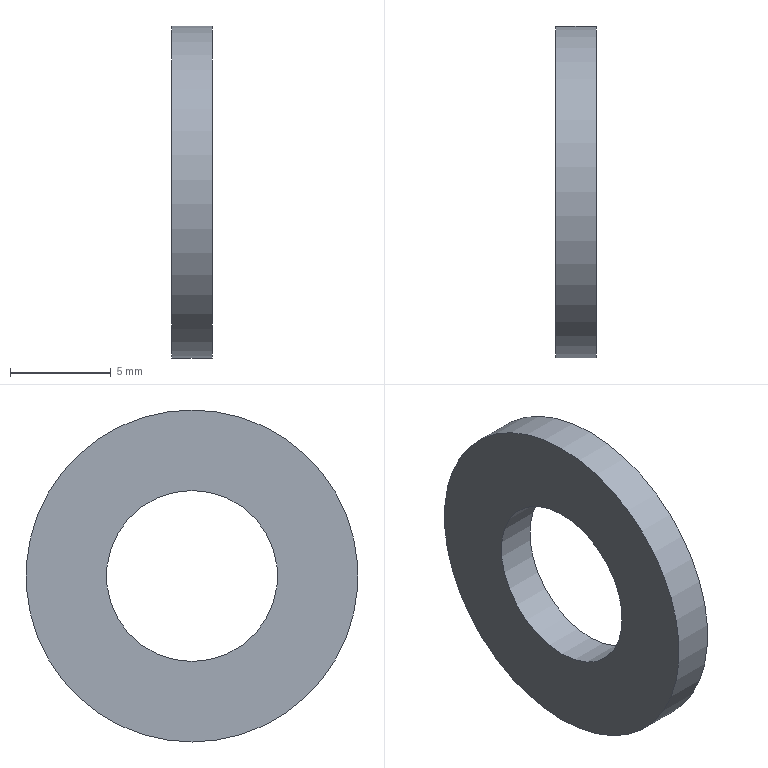Part | NX | features solid 2 | 1 solid | 4 faces | box 2 x 16.5 x 16.5 mm | volume 314.159 mm3 | plane 2 | cylinder 2 | commonest cylinder face diameters 8.5 x1 16.5 x1
STEP:
#1=CARTESIAN_POINT('',(-277.,-465.,-88.75));
#2=VERTEX_POINT('',#1);
#3=CARTESIAN_POINT('',(-277.,-465.,-97.));
#4=DIRECTION('',(1.,0.,0.));
#5=DIRECTION('',(0.,0.,1.));
#6=AXIS2_PLACEMENT_3D('',#3,#4,#5);
#7=CIRCLE('',#6,8.25);
#8=EDGE_CURVE('',#2,#2,#7,.F.);
#9=ORIENTED_EDGE('',*,*,#8,.T.);
#10=EDGE_LOOP('',(#9));
#11=FACE_BOUND('',#10,.T.);
#12=CARTESIAN_POINT('',(-277.,-465.,-101.25));
#13=VERTEX_POINT('',#12);
#14=CARTESIAN_POINT('',(-277.,-465.,-97.));
#15=DIRECTION('',(-1.,0.,0.));
#16=DIRECTION('',(0.,0.,-1.));
#17=AXIS2_PLACEMENT_3D('',#14,#15,#16);
#18=CIRCLE('',#17,4.25);
#19=EDGE_CURVE('',#13,#13,#18,.T.);
#20=ORIENTED_EDGE('',*,*,#19,.F.);
#21=EDGE_LOOP('',(#20));
#22=FACE_BOUND('',#21,.T.);
#23=CARTESIAN_POINT('',(-277.,-465.,-97.));
#24=DIRECTION('',(-1.,0.,0.));
#25=DIRECTION('',(0.,0.,1.));
#26=AXIS2_PLACEMENT_3D('',#23,#24,#25);
#27=PLANE('',#26);
#28=ADVANCED_FACE('',(#11,#22),#27,.T.);
#29=CARTESIAN_POINT('',(-275.,-465.,-88.75));
#30=VERTEX_POINT('',#29);
#31=CARTESIAN_POINT('',(-275.,-465.,-97.));
#32=DIRECTION('',(1.,0.,0.));
#33=DIRECTION('',(0.,0.,1.));
#34=AXIS2_PLACEMENT_3D('',#31,#32,#33);
#35=CIRCLE('',#34,8.25);
#36=EDGE_CURVE('',#30,#30,#35,.F.);
#37=ORIENTED_EDGE('',*,*,#36,.F.);
#38=EDGE_LOOP('',(#37));
#39=FACE_BOUND('',#38,.T.);
#40=CARTESIAN_POINT('',(-275.,-465.,-101.25));
#41=VERTEX_POINT('',#40);
#42=CARTESIAN_POINT('',(-275.,-465.,-97.));
#43=DIRECTION('',(-1.,0.,0.));
#44=DIRECTION('',(0.,0.,-1.));
#45=AXIS2_PLACEMENT_3D('',#42,#43,#44);
#46=CIRCLE('',#45,4.25);
#47=EDGE_CURVE('',#41,#41,#46,.T.);
#48=ORIENTED_EDGE('',*,*,#47,.T.);
#49=EDGE_LOOP('',(#48));
#50=FACE_BOUND('',#49,.T.);
#51=CARTESIAN_POINT('',(-275.,-465.,-97.));
#52=DIRECTION('',(-1.,0.,0.));
#53=DIRECTION('',(0.,0.,1.));
#54=AXIS2_PLACEMENT_3D('',#51,#52,#53);
#55=PLANE('',#54);
#56=ADVANCED_FACE('',(#39,#50),#55,.F.);
#57=ORIENTED_EDGE('',*,*,#8,.F.);
#58=EDGE_LOOP('',(#57));
#59=FACE_BOUND('',#58,.T.);
#60=ORIENTED_EDGE('',*,*,#36,.T.);
#61=EDGE_LOOP('',(#60));
#62=FACE_BOUND('',#61,.T.);
#63=CARTESIAN_POINT('',(-275.,-465.,-97.));
#64=DIRECTION('',(-1.,0.,0.));
#65=DIRECTION('',(0.,0.,1.));
#66=AXIS2_PLACEMENT_3D('',#63,#64,#65);
#67=CYLINDRICAL_SURFACE('',#66,8.25);
#68=ADVANCED_FACE('',(#59,#62),#67,.T.);
#69=ORIENTED_EDGE('',*,*,#19,.T.);
#70=EDGE_LOOP('',(#69));
#71=FACE_BOUND('',#70,.T.);
#72=ORIENTED_EDGE('',*,*,#47,.F.);
#73=EDGE_LOOP('',(#72));
#74=FACE_BOUND('',#73,.T.);
#75=CARTESIAN_POINT('',(-275.,-465.,-97.));
#76=DIRECTION('',(-1.,0.,0.));
#77=DIRECTION('',(0.,0.,1.));
#78=AXIS2_PLACEMENT_3D('',#75,#76,#77);
#79=CYLINDRICAL_SURFACE('',#78,4.25);
#80=ADVANCED_FACE('',(#71,#74),#79,.F.);
#81=CLOSED_SHELL('',(#28,#56,#68,#80));
#82=MANIFOLD_SOLID_BREP('',#81);
#83=(LENGTH_UNIT()NAMED_UNIT(*)SI_UNIT(.MILLI.,.METRE.));
#84=UNCERTAINTY_MEASURE_WITH_UNIT(LENGTH_MEASURE(0.00001),#83,'','');
#85=(NAMED_UNIT(*)PLANE_ANGLE_UNIT()SI_UNIT($,.RADIAN.));
#86=(NAMED_UNIT(*)SI_UNIT($,.STERADIAN.)SOLID_ANGLE_UNIT());
#87=(GEOMETRIC_REPRESENTATION_CONTEXT(3)GLOBAL_UNCERTAINTY_ASSIGNED_CONTEXT((#84))GLOBAL_UNIT_ASSIGNED_CONTEXT((#83,#85,#86))REPRESENTATION_CONTEXT('',''));
#88=ADVANCED_BREP_SHAPE_REPRESENTATION('',(#82),#87);